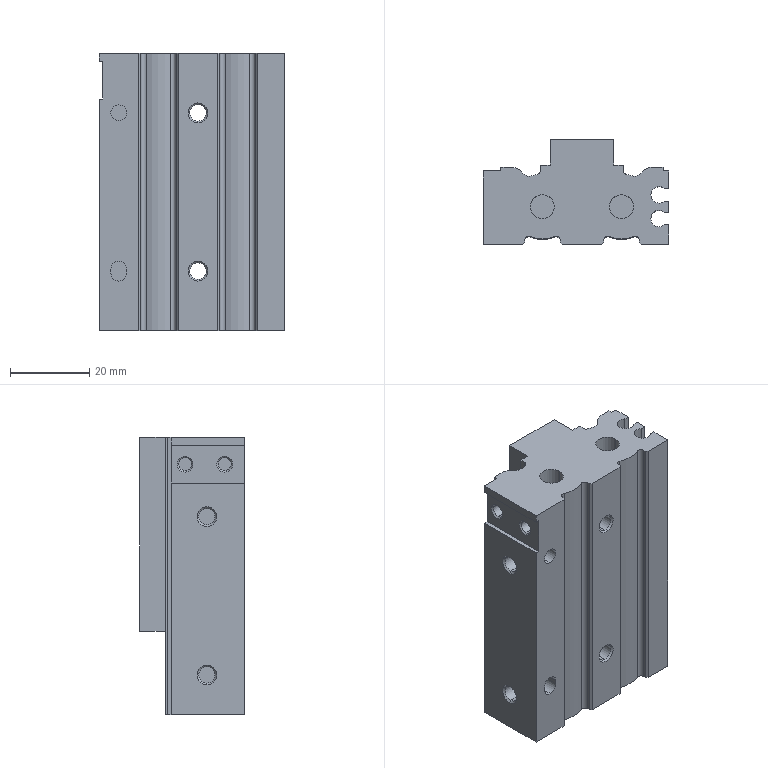Part | SolidWorks | features BaseBody 1 | 1 solid | 138 faces | box 47 x 26.5 x 70 mm | volume 54767 mm3 | plane 61 | cylinder 57 | cone 20 | commonest cylinder face diameters 3.242 x12 4.2 x8 4 x7 2 x6 4.134 x4 6 x4